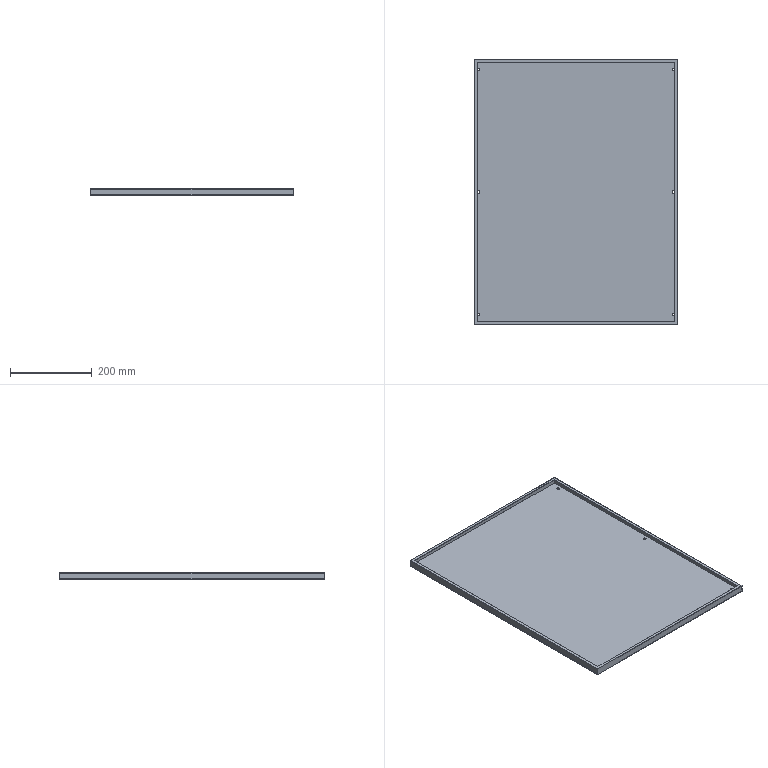Part | STEP file | 1 solid | 28 faces | box 498 x 650 x 17.5 mm | volume 560596 mm3 | plane 16 | cylinder 12 | commonest cylinder face diameters 6 x12